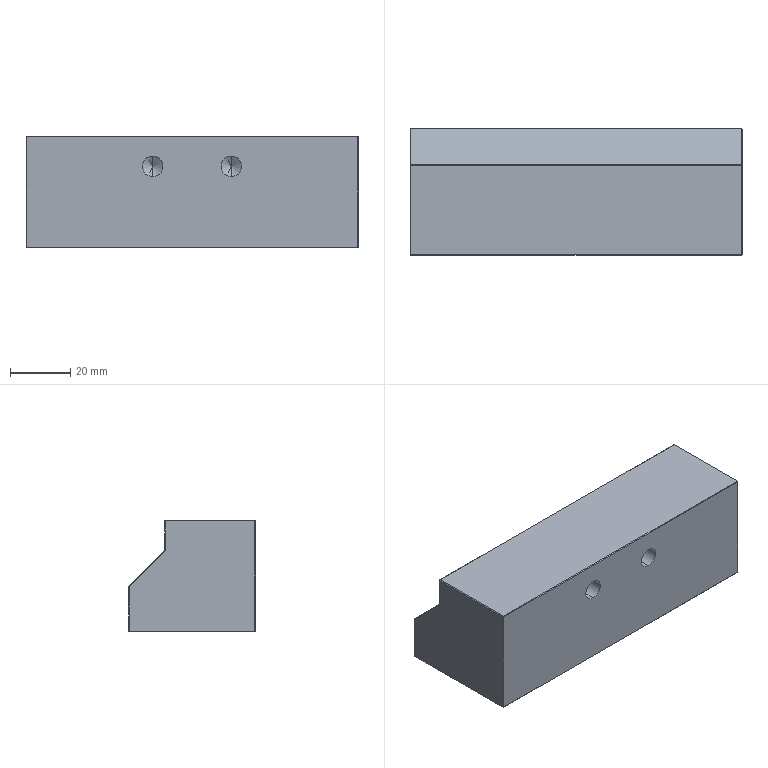Part | 1 solid | 40 faces | box 110 x 42 x 37 mm | volume 148303 mm3 | plane 32 | cylinder 4 | cone 4 | commonest cylinder face diameters 6.8 x4
STEP:
#1=CARTESIAN_POINT('',(-13.,20.,9.4));
#2=VERTEX_POINT('',#1);
#3=CARTESIAN_POINT('',(-13.,20.,2.6));
#4=VERTEX_POINT('',#3);
#5=CARTESIAN_POINT('',(-13.,20.,6.));
#6=DIRECTION('',(0.,-1.,0.));
#7=DIRECTION('',(0.,0.,-1.));
#8=AXIS2_PLACEMENT_3D('',#5,#6,#7);
#9=CIRCLE('',#8,3.4);
#10=EDGE_CURVE('',#2,#4,#9,.T.);
#11=ORIENTED_EDGE('',*,*,#10,.F.);
#12=CARTESIAN_POINT('',(-13.,0.,9.4));
#13=VERTEX_POINT('',#12);
#14=CARTESIAN_POINT('',(-13.,0.,9.4));
#15=DIRECTION('',(0.,-1.,0.));
#16=VECTOR('',#15,1000.);
#17=LINE('',#14,#16);
#18=EDGE_CURVE('',#2,#13,#17,.T.);
#19=ORIENTED_EDGE('',*,*,#18,.T.);
#20=CARTESIAN_POINT('',(-13.,0.,2.6));
#21=VERTEX_POINT('',#20);
#22=CARTESIAN_POINT('',(-13.,0.,6.));
#23=DIRECTION('',(0.,-1.,0.));
#24=DIRECTION('',(0.,0.,-1.));
#25=AXIS2_PLACEMENT_3D('',#22,#23,#24);
#26=CIRCLE('',#25,3.4);
#27=EDGE_CURVE('',#13,#21,#26,.T.);
#28=ORIENTED_EDGE('',*,*,#27,.T.);
#29=CARTESIAN_POINT('',(-13.,0.,2.6));
#30=DIRECTION('',(0.,-1.,0.));
#31=VECTOR('',#30,1000.);
#32=LINE('',#29,#31);
#33=EDGE_CURVE('',#4,#21,#32,.T.);
#34=ORIENTED_EDGE('',*,*,#33,.F.);
#35=EDGE_LOOP('',(#11,#19,#28,#34));
#36=FACE_OUTER_BOUND('',#35,.T.);
#37=CARTESIAN_POINT('',(-13.,0.,6.));
#38=DIRECTION('',(0.,-1.,0.));
#39=DIRECTION('',(0.,0.,-1.));
#40=AXIS2_PLACEMENT_3D('',#37,#38,#39);
#41=CYLINDRICAL_SURFACE('',#40,3.4);
#42=ADVANCED_FACE('',(#36),#41,.F.);
#43=CARTESIAN_POINT('',(-13.,22.043,6.));
#44=VERTEX_POINT('',#43);
#45=CARTESIAN_POINT('',(-13.,20.,2.6));
#46=DIRECTION('',(0.,-0.515,-0.8572));
#47=VECTOR('',#46,1000.);
#48=LINE('',#45,#47);
#49=EDGE_CURVE('',#44,#4,#48,.T.);
#50=ORIENTED_EDGE('',*,*,#49,.F.);
#51=CARTESIAN_POINT('',(-13.,20.,9.4));
#52=DIRECTION('',(0.,-0.515,0.8572));
#53=VECTOR('',#52,1000.);
#54=LINE('',#51,#53);
#55=EDGE_CURVE('',#44,#2,#54,.T.);
#56=ORIENTED_EDGE('',*,*,#55,.T.);
#57=ORIENTED_EDGE('',*,*,#10,.T.);
#58=EDGE_LOOP('',(#50,#56,#57));
#59=FACE_OUTER_BOUND('',#58,.T.);
#60=CARTESIAN_POINT('',(-13.,20.,6.));
#61=DIRECTION('',(0.,-1.,0.));
#62=DIRECTION('',(0.,0.,-1.));
#63=AXIS2_PLACEMENT_3D('',#60,#61,#62);
#64=CONICAL_SURFACE('',#63,3.4,1.03);
#65=ADVANCED_FACE('',(#59),#64,.F.);
#66=CARTESIAN_POINT('',(13.,20.,9.4));
#67=VERTEX_POINT('',#66);
#68=CARTESIAN_POINT('',(13.,20.,2.6));
#69=VERTEX_POINT('',#68);
#70=CARTESIAN_POINT('',(13.,20.,6.));
#71=DIRECTION('',(0.,-1.,0.));
#72=DIRECTION('',(0.,0.,-1.));
#73=AXIS2_PLACEMENT_3D('',#70,#71,#72);
#74=CIRCLE('',#73,3.4);
#75=EDGE_CURVE('',#67,#69,#74,.T.);
#76=ORIENTED_EDGE('',*,*,#75,.F.);
#77=CARTESIAN_POINT('',(13.,0.,9.4));
#78=VERTEX_POINT('',#77);
#79=CARTESIAN_POINT('',(13.,0.,9.4));
#80=DIRECTION('',(0.,-1.,0.));
#81=VECTOR('',#80,1000.);
#82=LINE('',#79,#81);
#83=EDGE_CURVE('',#67,#78,#82,.T.);
#84=ORIENTED_EDGE('',*,*,#83,.T.);
#85=CARTESIAN_POINT('',(13.,0.,2.6));
#86=VERTEX_POINT('',#85);
#87=CARTESIAN_POINT('',(13.,0.,6.));
#88=DIRECTION('',(0.,-1.,0.));
#89=DIRECTION('',(0.,0.,-1.));
#90=AXIS2_PLACEMENT_3D('',#87,#88,#89);
#91=CIRCLE('',#90,3.4);
#92=EDGE_CURVE('',#78,#86,#91,.T.);
#93=ORIENTED_EDGE('',*,*,#92,.T.);
#94=CARTESIAN_POINT('',(13.,0.,2.6));
#95=DIRECTION('',(0.,-1.,0.));
#96=VECTOR('',#95,1000.);
#97=LINE('',#94,#96);
#98=EDGE_CURVE('',#69,#86,#97,.T.);
#99=ORIENTED_EDGE('',*,*,#98,.F.);
#100=EDGE_LOOP('',(#76,#84,#93,#99));
#101=FACE_OUTER_BOUND('',#100,.T.);
#102=CARTESIAN_POINT('',(13.,0.,6.));
#103=DIRECTION('',(0.,-1.,0.));
#104=DIRECTION('',(0.,0.,-1.));
#105=AXIS2_PLACEMENT_3D('',#102,#103,#104);
#106=CYLINDRICAL_SURFACE('',#105,3.4);
#107=ADVANCED_FACE('',(#101),#106,.F.);
#108=CARTESIAN_POINT('',(13.,22.043,6.));
#109=VERTEX_POINT('',#108);
#110=CARTESIAN_POINT('',(13.,20.,2.6));
#111=DIRECTION('',(0.,-0.515,-0.8572));
#112=VECTOR('',#111,1000.);
#113=LINE('',#110,#112);
#114=EDGE_CURVE('',#109,#69,#113,.T.);
#115=ORIENTED_EDGE('',*,*,#114,.F.);
#116=CARTESIAN_POINT('',(13.,20.,9.4));
#117=DIRECTION('',(0.,-0.515,0.8572));
#118=VECTOR('',#117,1000.);
#119=LINE('',#116,#118);
#120=EDGE_CURVE('',#109,#67,#119,.T.);
#121=ORIENTED_EDGE('',*,*,#120,.T.);
#122=ORIENTED_EDGE('',*,*,#75,.T.);
#123=EDGE_LOOP('',(#115,#121,#122));
#124=FACE_OUTER_BOUND('',#123,.T.);
#125=CARTESIAN_POINT('',(13.,20.,6.));
#126=DIRECTION('',(0.,-1.,0.));
#127=DIRECTION('',(0.,0.,-1.));
#128=AXIS2_PLACEMENT_3D('',#125,#126,#127);
#129=CONICAL_SURFACE('',#128,3.4,1.03);
#130=ADVANCED_FACE('',(#124),#129,.F.);
#131=CARTESIAN_POINT('',(-54.8,0.,15.8));
#132=VERTEX_POINT('',#131);
#133=CARTESIAN_POINT('',(-54.8,0.,-20.8));
#134=VERTEX_POINT('',#133);
#135=CARTESIAN_POINT('',(-54.8,0.,10.));
#136=DIRECTION('',(0.,0.,-1.));
#137=VECTOR('',#136,1000.);
#138=LINE('',#135,#137);
#139=EDGE_CURVE('',#132,#134,#138,.T.);
#140=ORIENTED_EDGE('',*,*,#139,.T.);
#141=CARTESIAN_POINT('',(54.8,0.,-20.8));
#142=VERTEX_POINT('',#141);
#143=CARTESIAN_POINT('',(55.,0.,-20.8));
#144=DIRECTION('',(1.,0.,0.));
#145=VECTOR('',#144,1000.);
#146=LINE('',#143,#145);
#147=EDGE_CURVE('',#134,#142,#146,.T.);
#148=ORIENTED_EDGE('',*,*,#147,.T.);
#149=CARTESIAN_POINT('',(54.8,0.,15.8));
#150=VERTEX_POINT('',#149);
#151=CARTESIAN_POINT('',(54.8,0.,16.));
#152=DIRECTION('',(0.,0.,1.));
#153=VECTOR('',#152,1000.);
#154=LINE('',#151,#153);
#155=EDGE_CURVE('',#142,#150,#154,.T.);
#156=ORIENTED_EDGE('',*,*,#155,.T.);
#157=CARTESIAN_POINT('',(55.,0.,15.8));
#158=DIRECTION('',(-1.,0.,0.));
#159=VECTOR('',#158,1000.);
#160=LINE('',#157,#159);
#161=EDGE_CURVE('',#150,#132,#160,.T.);
#162=ORIENTED_EDGE('',*,*,#161,.T.);
#163=EDGE_LOOP('',(#140,#148,#156,#162));
#164=FACE_OUTER_BOUND('',#163,.T.);
#165=CARTESIAN_POINT('',(-13.,0.,6.));
#166=DIRECTION('',(0.,-1.,0.));
#167=DIRECTION('',(0.,0.,-1.));
#168=AXIS2_PLACEMENT_3D('',#165,#166,#167);
#169=CIRCLE('',#168,3.4);
#170=EDGE_CURVE('',#21,#13,#169,.T.);
#171=ORIENTED_EDGE('',*,*,#170,.F.);
#172=ORIENTED_EDGE('',*,*,#27,.F.);
#173=EDGE_LOOP('',(#171,#172));
#174=FACE_BOUND('',#173,.T.);
#175=CARTESIAN_POINT('',(13.,0.,6.));
#176=DIRECTION('',(0.,-1.,0.));
#177=DIRECTION('',(0.,0.,-1.));
#178=AXIS2_PLACEMENT_3D('',#175,#176,#177);
#179=CIRCLE('',#178,3.4);
#180=EDGE_CURVE('',#86,#78,#179,.T.);
#181=ORIENTED_EDGE('',*,*,#180,.F.);
#182=ORIENTED_EDGE('',*,*,#92,.F.);
#183=EDGE_LOOP('',(#181,#182));
#184=FACE_BOUND('',#183,.T.);
#185=CARTESIAN_POINT('',(55.,0.,10.));
#186=DIRECTION('',(0.,1.,0.));
#187=DIRECTION('',(0.,0.,1.));
#188=AXIS2_PLACEMENT_3D('',#185,#186,#187);
#189=PLANE('',#188);
#190=ADVANCED_FACE('',(#164,#174,#184),#189,.F.);
#191=CARTESIAN_POINT('',(-54.8,41.8,-21.));
#192=VERTEX_POINT('',#191);
#193=CARTESIAN_POINT('',(54.8,41.8,-21.));
#194=VERTEX_POINT('',#193);
#195=CARTESIAN_POINT('',(55.,41.8,-21.));
#196=DIRECTION('',(1.,0.,0.));
#197=VECTOR('',#196,1000.);
#198=LINE('',#195,#197);
#199=EDGE_CURVE('',#192,#194,#198,.T.);
#200=ORIENTED_EDGE('',*,*,#199,.T.);
#201=CARTESIAN_POINT('',(54.8,0.2,-21.));
#202=VERTEX_POINT('',#201);
#203=CARTESIAN_POINT('',(54.8,0.,-21.));
#204=DIRECTION('',(0.,-1.,0.));
#205=VECTOR('',#204,1000.);
#206=LINE('',#203,#205);
#207=EDGE_CURVE('',#194,#202,#206,.T.);
#208=ORIENTED_EDGE('',*,*,#207,.T.);
#209=CARTESIAN_POINT('',(-54.8,0.2,-21.));
#210=VERTEX_POINT('',#209);
#211=CARTESIAN_POINT('',(55.,0.2,-21.));
#212=DIRECTION('',(-1.,0.,0.));
#213=VECTOR('',#212,1000.);
#214=LINE('',#211,#213);
#215=EDGE_CURVE('',#202,#210,#214,.T.);
#216=ORIENTED_EDGE('',*,*,#215,.T.);
#217=CARTESIAN_POINT('',(-54.8,0.,-21.));
#218=DIRECTION('',(0.,1.,0.));
#219=VECTOR('',#218,1000.);
#220=LINE('',#217,#219);
#221=EDGE_CURVE('',#210,#192,#220,.T.);
#222=ORIENTED_EDGE('',*,*,#221,.T.);
#223=EDGE_LOOP('',(#200,#208,#216,#222));
#224=FACE_OUTER_BOUND('',#223,.T.);
#225=CARTESIAN_POINT('',(55.,0.,-21.));
#226=DIRECTION('',(0.,0.,1.));
#227=DIRECTION('',(1.,0.,0.));
#228=AXIS2_PLACEMENT_3D('',#225,#226,#227);
#229=PLANE('',#228);
#230=ADVANCED_FACE('',(#224),#229,.F.);
#231=CARTESIAN_POINT('',(54.8,42.,-6.));
#232=VERTEX_POINT('',#231);
#233=CARTESIAN_POINT('',(-54.8,42.,-6.));
#234=VERTEX_POINT('',#233);
#235=CARTESIAN_POINT('',(55.,42.,-6.));
#236=DIRECTION('',(-1.,0.,0.));
#237=VECTOR('',#236,1000.);
#238=LINE('',#235,#237);
#239=EDGE_CURVE('',#232,#234,#238,.T.);
#240=ORIENTED_EDGE('',*,*,#239,.F.);
#241=CARTESIAN_POINT('',(54.8,42.,-20.8));
#242=VERTEX_POINT('',#241);
#243=CARTESIAN_POINT('',(54.8,42.,-21.));
#244=DIRECTION('',(0.,0.,-1.));
#245=VECTOR('',#244,1000.);
#246=LINE('',#243,#245);
#247=EDGE_CURVE('',#232,#242,#246,.T.);
#248=ORIENTED_EDGE('',*,*,#247,.T.);
#249=CARTESIAN_POINT('',(-54.8,42.,-20.8));
#250=VERTEX_POINT('',#249);
#251=CARTESIAN_POINT('',(55.,42.,-20.8));
#252=DIRECTION('',(-1.,0.,0.));
#253=VECTOR('',#252,1000.);
#254=LINE('',#251,#253);
#255=EDGE_CURVE('',#242,#250,#254,.T.);
#256=ORIENTED_EDGE('',*,*,#255,.T.);
#257=CARTESIAN_POINT('',(-54.8,42.,-21.));
#258=DIRECTION('',(0.,0.,1.));
#259=VECTOR('',#258,1000.);
#260=LINE('',#257,#259);
#261=EDGE_CURVE('',#250,#234,#260,.T.);
#262=ORIENTED_EDGE('',*,*,#261,.T.);
#263=EDGE_LOOP('',(#240,#248,#256,#262));
#264=FACE_OUTER_BOUND('',#263,.T.);
#265=CARTESIAN_POINT('',(55.,42.,-21.));
#266=DIRECTION('',(0.,-1.,0.));
#267=DIRECTION('',(0.,0.,-1.));
#268=AXIS2_PLACEMENT_3D('',#265,#266,#267);
#269=PLANE('',#268);
#270=ADVANCED_FACE('',(#264),#269,.F.);
#271=CARTESIAN_POINT('',(54.8,30.,6.));
#272=VERTEX_POINT('',#271);
#273=CARTESIAN_POINT('',(-54.8,30.,6.));
#274=VERTEX_POINT('',#273);
#275=CARTESIAN_POINT('',(55.,30.,6.));
#276=DIRECTION('',(-1.,0.,0.));
#277=VECTOR('',#276,1000.);
#278=LINE('',#275,#277);
#279=EDGE_CURVE('',#272,#274,#278,.T.);
#280=ORIENTED_EDGE('',*,*,#279,.F.);
#281=CARTESIAN_POINT('',(54.8,42.,-6.));
#282=DIRECTION('',(0.,0.7071,-0.7071));
#283=VECTOR('',#282,1000.);
#284=LINE('',#281,#283);
#285=EDGE_CURVE('',#272,#232,#284,.T.);
#286=ORIENTED_EDGE('',*,*,#285,.T.);
#287=ORIENTED_EDGE('',*,*,#239,.T.);
#288=CARTESIAN_POINT('',(-54.8,42.,-6.));
#289=DIRECTION('',(0.,-0.7071,0.7071));
#290=VECTOR('',#289,1000.);
#291=LINE('',#288,#290);
#292=EDGE_CURVE('',#234,#274,#291,.T.);
#293=ORIENTED_EDGE('',*,*,#292,.T.);
#294=EDGE_LOOP('',(#280,#286,#287,#293));
#295=FACE_OUTER_BOUND('',#294,.T.);
#296=CARTESIAN_POINT('',(55.,42.,-6.));
#297=DIRECTION('',(0.,-0.7071,-0.7071));
#298=DIRECTION('',(0.,0.7071,-0.7071));
#299=AXIS2_PLACEMENT_3D('',#296,#297,#298);
#300=PLANE('',#299);
#301=ADVANCED_FACE('',(#295),#300,.F.);
#302=CARTESIAN_POINT('',(-54.8,30.,15.8));
#303=VERTEX_POINT('',#302);
#304=CARTESIAN_POINT('',(54.8,30.,15.8));
#305=VERTEX_POINT('',#304);
#306=CARTESIAN_POINT('',(55.,30.,15.8));
#307=DIRECTION('',(1.,0.,0.));
#308=VECTOR('',#307,1000.);
#309=LINE('',#306,#308);
#310=EDGE_CURVE('',#303,#305,#309,.T.);
#311=ORIENTED_EDGE('',*,*,#310,.T.);
#312=CARTESIAN_POINT('',(54.8,30.,6.));
#313=DIRECTION('',(0.,0.,-1.));
#314=VECTOR('',#313,1000.);
#315=LINE('',#312,#314);
#316=EDGE_CURVE('',#305,#272,#315,.T.);
#317=ORIENTED_EDGE('',*,*,#316,.T.);
#318=ORIENTED_EDGE('',*,*,#279,.T.);
#319=CARTESIAN_POINT('',(-54.8,30.,6.));
#320=DIRECTION('',(0.,0.,1.));
#321=VECTOR('',#320,1000.);
#322=LINE('',#319,#321);
#323=EDGE_CURVE('',#274,#303,#322,.T.);
#324=ORIENTED_EDGE('',*,*,#323,.T.);
#325=EDGE_LOOP('',(#311,#317,#318,#324));
#326=FACE_OUTER_BOUND('',#325,.T.);
#327=CARTESIAN_POINT('',(55.,30.,6.));
#328=DIRECTION('',(0.,-1.,0.));
#329=DIRECTION('',(0.,0.,-1.));
#330=AXIS2_PLACEMENT_3D('',#327,#328,#329);
#331=PLANE('',#330);
#332=ADVANCED_FACE('',(#326),#331,.F.);
#333=CARTESIAN_POINT('',(54.8,0.2,16.));
#334=VERTEX_POINT('',#333);
#335=CARTESIAN_POINT('',(54.8,29.8,16.));
#336=VERTEX_POINT('',#335);
#337=CARTESIAN_POINT('',(54.8,30.,16.));
#338=DIRECTION('',(0.,1.,0.));
#339=VECTOR('',#338,1000.);
#340=LINE('',#337,#339);
#341=EDGE_CURVE('',#334,#336,#340,.T.);
#342=ORIENTED_EDGE('',*,*,#341,.T.);
#343=CARTESIAN_POINT('',(-54.8,29.8,16.));
#344=VERTEX_POINT('',#343);
#345=CARTESIAN_POINT('',(55.,29.8,16.));
#346=DIRECTION('',(-1.,0.,0.));
#347=VECTOR('',#346,1000.);
#348=LINE('',#345,#347);
#349=EDGE_CURVE('',#336,#344,#348,.T.);
#350=ORIENTED_EDGE('',*,*,#349,.T.);
#351=CARTESIAN_POINT('',(-54.8,0.2,16.));
#352=VERTEX_POINT('',#351);
#353=CARTESIAN_POINT('',(-54.8,30.,16.));
#354=DIRECTION('',(0.,-1.,0.));
#355=VECTOR('',#354,1000.);
#356=LINE('',#353,#355);
#357=EDGE_CURVE('',#344,#352,#356,.T.);
#358=ORIENTED_EDGE('',*,*,#357,.T.);
#359=CARTESIAN_POINT('',(55.,0.2,16.));
#360=DIRECTION('',(1.,0.,0.));
#361=VECTOR('',#360,1000.);
#362=LINE('',#359,#361);
#363=EDGE_CURVE('',#352,#334,#362,.T.);
#364=ORIENTED_EDGE('',*,*,#363,.T.);
#365=EDGE_LOOP('',(#342,#350,#358,#364));
#366=FACE_OUTER_BOUND('',#365,.T.);
#367=CARTESIAN_POINT('',(55.,30.,16.));
#368=DIRECTION('',(0.,0.,-1.));
#369=DIRECTION('',(0.,1.,0.));
#370=AXIS2_PLACEMENT_3D('',#367,#368,#369);
#371=PLANE('',#370);
#372=ADVANCED_FACE('',(#366),#371,.F.);
#373=CARTESIAN_POINT('',(55.,29.8,5.917));
#374=VERTEX_POINT('',#373);
#375=CARTESIAN_POINT('',(55.,29.8,15.8));
#376=VERTEX_POINT('',#375);
#377=CARTESIAN_POINT('',(55.,29.8,16.));
#378=DIRECTION('',(0.,0.,1.));
#379=VECTOR('',#378,1000.);
#380=LINE('',#377,#379);
#381=EDGE_CURVE('',#374,#376,#380,.T.);
#382=ORIENTED_EDGE('',*,*,#381,.T.);
#383=CARTESIAN_POINT('',(55.,0.2,15.8));
#384=VERTEX_POINT('',#383);
#385=CARTESIAN_POINT('',(55.,0.,15.8));
#386=DIRECTION('',(0.,-1.,0.));
#387=VECTOR('',#386,1000.);
#388=LINE('',#385,#387);
#389=EDGE_CURVE('',#376,#384,#388,.T.);
#390=ORIENTED_EDGE('',*,*,#389,.T.);
#391=CARTESIAN_POINT('',(55.,0.2,-20.8));
#392=VERTEX_POINT('',#391);
#393=CARTESIAN_POINT('',(55.,0.2,-21.));
#394=DIRECTION('',(0.,0.,-1.));
#395=VECTOR('',#394,1000.);
#396=LINE('',#393,#395);
#397=EDGE_CURVE('',#384,#392,#396,.T.);
#398=ORIENTED_EDGE('',*,*,#397,.T.);
#399=CARTESIAN_POINT('',(55.,41.8,-20.8));
#400=VERTEX_POINT('',#399);
#401=CARTESIAN_POINT('',(55.,42.,-20.8));
#402=DIRECTION('',(0.,1.,0.));
#403=VECTOR('',#402,1000.);
#404=LINE('',#401,#403);
#405=EDGE_CURVE('',#392,#400,#404,.T.);
#406=ORIENTED_EDGE('',*,*,#405,.T.);
#407=CARTESIAN_POINT('',(55.,41.8,-6.083));
#408=VERTEX_POINT('',#407);
#409=CARTESIAN_POINT('',(55.,41.8,-6.));
#410=DIRECTION('',(0.,0.,1.));
#411=VECTOR('',#410,1000.);
#412=LINE('',#409,#411);
#413=EDGE_CURVE('',#400,#408,#412,.T.);
#414=ORIENTED_EDGE('',*,*,#413,.T.);
#415=CARTESIAN_POINT('',(55.,29.859,5.859));
#416=DIRECTION('',(0.,-0.7071,0.7071));
#417=VECTOR('',#416,1000.);
#418=LINE('',#415,#417);
#419=EDGE_CURVE('',#408,#374,#418,.T.);
#420=ORIENTED_EDGE('',*,*,#419,.T.);
#421=EDGE_LOOP('',(#382,#390,#398,#406,#414,#420));
#422=FACE_OUTER_BOUND('',#421,.T.);
#423=CARTESIAN_POINT('',(55.,0.,0.));
#424=DIRECTION('',(1.,0.,0.));
#425=DIRECTION('',(0.,0.,-1.));
#426=AXIS2_PLACEMENT_3D('',#423,#424,#425);
#427=PLANE('',#426);
#428=ADVANCED_FACE('',(#422),#427,.T.);
#429=CARTESIAN_POINT('',(-55.,0.2,-20.8));
#430=VERTEX_POINT('',#429);
#431=CARTESIAN_POINT('',(-55.,0.2,15.8));
#432=VERTEX_POINT('',#431);
#433=CARTESIAN_POINT('',(-55.,0.2,0.));
#434=DIRECTION('',(0.,0.,1.));
#435=VECTOR('',#434,1000.);
#436=LINE('',#433,#435);
#437=EDGE_CURVE('',#430,#432,#436,.T.);
#438=ORIENTED_EDGE('',*,*,#437,.T.);
#439=CARTESIAN_POINT('',(-55.,29.8,15.8));
#440=VERTEX_POINT('',#439);
#441=CARTESIAN_POINT('',(-55.,0.,15.8));
#442=DIRECTION('',(0.,1.,0.));
#443=VECTOR('',#442,1000.);
#444=LINE('',#441,#443);
#445=EDGE_CURVE('',#432,#440,#444,.T.);
#446=ORIENTED_EDGE('',*,*,#445,.T.);
#447=CARTESIAN_POINT('',(-55.,29.8,5.917));
#448=VERTEX_POINT('',#447);
#449=CARTESIAN_POINT('',(-55.,29.8,0.));
#450=DIRECTION('',(0.,0.,-1.));
#451=VECTOR('',#450,1000.);
#452=LINE('',#449,#451);
#453=EDGE_CURVE('',#440,#448,#452,.T.);
#454=ORIENTED_EDGE('',*,*,#453,.T.);
#455=CARTESIAN_POINT('',(-55.,41.8,-6.083));
#456=VERTEX_POINT('',#455);
#457=CARTESIAN_POINT('',(-55.,17.859,17.859));
#458=DIRECTION('',(0.,0.7071,-0.7071));
#459=VECTOR('',#458,1000.);
#460=LINE('',#457,#459);
#461=EDGE_CURVE('',#448,#456,#460,.T.);
#462=ORIENTED_EDGE('',*,*,#461,.T.);
#463=CARTESIAN_POINT('',(-55.,41.8,-20.8));
#464=VERTEX_POINT('',#463);
#465=CARTESIAN_POINT('',(-55.,41.8,0.));
#466=DIRECTION('',(0.,0.,-1.));
#467=VECTOR('',#466,1000.);
#468=LINE('',#465,#467);
#469=EDGE_CURVE('',#456,#464,#468,.T.);
#470=ORIENTED_EDGE('',*,*,#469,.T.);
#471=CARTESIAN_POINT('',(-55.,0.,-20.8));
#472=DIRECTION('',(0.,-1.,0.));
#473=VECTOR('',#472,1000.);
#474=LINE('',#471,#473);
#475=EDGE_CURVE('',#464,#430,#474,.T.);
#476=ORIENTED_EDGE('',*,*,#475,.T.);
#477=EDGE_LOOP('',(#438,#446,#454,#462,#470,#476));
#478=FACE_OUTER_BOUND('',#477,.T.);
#479=CARTESIAN_POINT('',(-55.,0.,0.));
#480=DIRECTION('',(1.,0.,0.));
#481=DIRECTION('',(0.,0.,-1.));
#482=AXIS2_PLACEMENT_3D('',#479,#480,#481);
#483=PLANE('',#482);
#484=ADVANCED_FACE('',(#478),#483,.F.);
#485=ORIENTED_EDGE('',*,*,#120,.F.);
#486=ORIENTED_EDGE('',*,*,#114,.T.);
#487=CARTESIAN_POINT('',(13.,20.,6.));
#488=DIRECTION('',(0.,-1.,0.));
#489=DIRECTION('',(0.,0.,-1.));
#490=AXIS2_PLACEMENT_3D('',#487,#488,#489);
#491=CIRCLE('',#490,3.4);
#492=EDGE_CURVE('',#69,#67,#491,.T.);
#493=ORIENTED_EDGE('',*,*,#492,.T.);
#494=EDGE_LOOP('',(#485,#486,#493));
#495=FACE_OUTER_BOUND('',#494,.T.);
#496=CARTESIAN_POINT('',(13.,20.,6.));
#497=DIRECTION('',(0.,-1.,0.));
#498=DIRECTION('',(0.,0.,-1.));
#499=AXIS2_PLACEMENT_3D('',#496,#497,#498);
#500=CONICAL_SURFACE('',#499,3.4,1.03);
#501=ADVANCED_FACE('',(#495),#500,.F.);
#502=ORIENTED_EDGE('',*,*,#83,.F.);
#503=ORIENTED_EDGE('',*,*,#492,.F.);
#504=ORIENTED_EDGE('',*,*,#98,.T.);
#505=ORIENTED_EDGE('',*,*,#180,.T.);
#506=EDGE_LOOP('',(#502,#503,#504,#505));
#507=FACE_OUTER_BOUND('',#506,.T.);
#508=CARTESIAN_POINT('',(13.,0.,6.));
#509=DIRECTION('',(0.,-1.,0.));
#510=DIRECTION('',(0.,0.,-1.));
#511=AXIS2_PLACEMENT_3D('',#508,#509,#510);
#512=CYLINDRICAL_SURFACE('',#511,3.4);
#513=ADVANCED_FACE('',(#507),#512,.F.);
#514=ORIENTED_EDGE('',*,*,#55,.F.);
#515=ORIENTED_EDGE('',*,*,#49,.T.);
#516=CARTESIAN_POINT('',(-13.,20.,6.));
#517=DIRECTION('',(0.,-1.,0.));
#518=DIRECTION('',(0.,0.,-1.));
#519=AXIS2_PLACEMENT_3D('',#516,#517,#518);
#520=CIRCLE('',#519,3.4);
#521=EDGE_CURVE('',#4,#2,#520,.T.);
#522=ORIENTED_EDGE('',*,*,#521,.T.);
#523=EDGE_LOOP('',(#514,#515,#522));
#524=FACE_OUTER_BOUND('',#523,.T.);
#525=CARTESIAN_POINT('',(-13.,20.,6.));
#526=DIRECTION('',(0.,-1.,0.));
#527=DIRECTION('',(0.,0.,-1.));
#528=AXIS2_PLACEMENT_3D('',#525,#526,#527);
#529=CONICAL_SURFACE('',#528,3.4,1.03);
#530=ADVANCED_FACE('',(#524),#529,.F.);
#531=ORIENTED_EDGE('',*,*,#18,.F.);
#532=ORIENTED_EDGE('',*,*,#521,.F.);
#533=ORIENTED_EDGE('',*,*,#33,.T.);
#534=ORIENTED_EDGE('',*,*,#170,.T.);
#535=EDGE_LOOP('',(#531,#532,#533,#534));
#536=FACE_OUTER_BOUND('',#535,.T.);
#537=CARTESIAN_POINT('',(-13.,0.,6.));
#538=DIRECTION('',(0.,-1.,0.));
#539=DIRECTION('',(0.,0.,-1.));
#540=AXIS2_PLACEMENT_3D('',#537,#538,#539);
#541=CYLINDRICAL_SURFACE('',#540,3.4);
#542=ADVANCED_FACE('',(#536),#541,.F.);
#543=CARTESIAN_POINT('',(56.129,28.671,5.45));
#544=DIRECTION('',(0.6786,-0.6786,-0.2811));
#545=VECTOR('',#544,1000.);
#546=LINE('',#543,#545);
#547=EDGE_CURVE('',#272,#374,#546,.T.);
#548=ORIENTED_EDGE('',*,*,#547,.F.);
#549=ORIENTED_EDGE('',*,*,#316,.F.);
#550=CARTESIAN_POINT('',(54.8,30.,15.8));
#551=DIRECTION('',(-0.7071,0.7071,0.));
#552=VECTOR('',#551,1000.);
#553=LINE('',#550,#552);
#554=EDGE_CURVE('',#376,#305,#553,.T.);
#555=ORIENTED_EDGE('',*,*,#554,.F.);
#556=ORIENTED_EDGE('',*,*,#381,.F.);
#557=EDGE_LOOP('',(#548,#549,#555,#556));
#558=FACE_OUTER_BOUND('',#557,.T.);
#559=CARTESIAN_POINT('',(55.,29.8,0.));
#560=DIRECTION('',(0.7071,0.7071,0.));
#561=DIRECTION('',(0.,0.,-1.));
#562=AXIS2_PLACEMENT_3D('',#559,#560,#561);
#563=PLANE('',#562);
#564=ADVANCED_FACE('',(#558),#563,.T.);
#565=CARTESIAN_POINT('',(-54.9,29.9,15.8));
#566=DIRECTION('',(-0.7071,-0.7071,0.));
#567=VECTOR('',#566,1000.);
#568=LINE('',#565,#567);
#569=EDGE_CURVE('',#303,#440,#568,.T.);
#570=ORIENTED_EDGE('',*,*,#569,.F.);
#571=ORIENTED_EDGE('',*,*,#323,.F.);
#572=CARTESIAN_POINT('',(-54.8,30.,6.));
#573=DIRECTION('',(0.6786,0.6786,0.2811));
#574=VECTOR('',#573,1000.);
#575=LINE('',#572,#574);
#576=EDGE_CURVE('',#448,#274,#575,.T.);
#577=ORIENTED_EDGE('',*,*,#576,.F.);
#578=ORIENTED_EDGE('',*,*,#453,.F.);
#579=EDGE_LOOP('',(#570,#571,#577,#578));
#580=FACE_OUTER_BOUND('',#579,.T.);
#581=CARTESIAN_POINT('',(-54.8,30.,6.));
#582=DIRECTION('',(0.7071,-0.7071,0.));
#583=DIRECTION('',(0.,0.,1.));
#584=AXIS2_PLACEMENT_3D('',#581,#582,#583);
#585=PLANE('',#584);
#586=ADVANCED_FACE('',(#580),#585,.F.);
#587=CARTESIAN_POINT('',(54.8,30.,15.8));
#588=DIRECTION('',(0.,-0.7071,0.7071));
#589=VECTOR('',#588,1000.);
#590=LINE('',#587,#589);
#591=EDGE_CURVE('',#305,#336,#590,.T.);
#592=ORIENTED_EDGE('',*,*,#591,.F.);
#593=ORIENTED_EDGE('',*,*,#310,.F.);
#594=CARTESIAN_POINT('',(-54.8,29.8,16.));
#595=DIRECTION('',(0.,0.7071,-0.7071));
#596=VECTOR('',#595,1000.);
#597=LINE('',#594,#596);
#598=EDGE_CURVE('',#344,#303,#597,.T.);
#599=ORIENTED_EDGE('',*,*,#598,.F.);
#600=ORIENTED_EDGE('',*,*,#349,.F.);
#601=EDGE_LOOP('',(#592,#593,#599,#600));
#602=FACE_OUTER_BOUND('',#601,.T.);
#603=CARTESIAN_POINT('',(55.,29.8,16.));
#604=DIRECTION('',(0.,-0.7071,-0.7071));
#605=DIRECTION('',(-1.,0.,0.));
#606=AXIS2_PLACEMENT_3D('',#603,#604,#605);
#607=PLANE('',#606);
#608=ADVANCED_FACE('',(#602),#607,.F.);
#609=ORIENTED_EDGE('',*,*,#554,.T.);
#610=ORIENTED_EDGE('',*,*,#591,.T.);
#611=CARTESIAN_POINT('',(54.9,29.8,15.9));
#612=DIRECTION('',(-0.7071,0.,0.7071));
#613=VECTOR('',#612,1000.);
#614=LINE('',#611,#613);
#615=EDGE_CURVE('',#376,#336,#614,.T.);
#616=ORIENTED_EDGE('',*,*,#615,.F.);
#617=EDGE_LOOP('',(#609,#610,#616));
#618=FACE_OUTER_BOUND('',#617,.T.);
#619=CARTESIAN_POINT('',(54.8,30.,15.8));
#620=DIRECTION('',(0.5774,0.5774,0.5774));
#621=DIRECTION('',(0.,-0.7071,0.7071));
#622=AXIS2_PLACEMENT_3D('',#619,#620,#621);
#623=PLANE('',#622);
#624=ADVANCED_FACE('',(#618),#623,.T.);
#625=ORIENTED_EDGE('',*,*,#547,.T.);
#626=ORIENTED_EDGE('',*,*,#419,.F.);
#627=CARTESIAN_POINT('',(53.84,42.96,-5.602));
#628=DIRECTION('',(0.6786,-0.6786,-0.2811));
#629=VECTOR('',#628,1000.);
#630=LINE('',#627,#629);
#631=EDGE_CURVE('',#232,#408,#630,.T.);
#632=ORIENTED_EDGE('',*,*,#631,.F.);
#633=ORIENTED_EDGE('',*,*,#285,.F.);
#634=EDGE_LOOP('',(#625,#626,#632,#633));
#635=FACE_OUTER_BOUND('',#634,.T.);
#636=CARTESIAN_POINT('',(55.,17.859,17.859));
#637=DIRECTION('',(0.7071,0.5,0.5));
#638=DIRECTION('',(0.,0.7071,-0.7071));
#639=AXIS2_PLACEMENT_3D('',#636,#637,#638);
#640=PLANE('',#639);
#641=ADVANCED_FACE('',(#635),#640,.T.);
#642=ORIENTED_EDGE('',*,*,#576,.T.);
#643=ORIENTED_EDGE('',*,*,#292,.F.);
#644=CARTESIAN_POINT('',(-57.661,39.139,-7.185));
#645=DIRECTION('',(0.6786,0.6786,0.2811));
#646=VECTOR('',#645,1000.);
#647=LINE('',#644,#646);
#648=EDGE_CURVE('',#456,#234,#647,.T.);
#649=ORIENTED_EDGE('',*,*,#648,.F.);
#650=ORIENTED_EDGE('',*,*,#461,.F.);
#651=EDGE_LOOP('',(#642,#643,#649,#650));
#652=FACE_OUTER_BOUND('',#651,.T.);
#653=CARTESIAN_POINT('',(-54.8,42.,-6.));
#654=DIRECTION('',(0.7071,-0.5,-0.5));
#655=DIRECTION('',(0.,-0.7071,0.7071));
#656=AXIS2_PLACEMENT_3D('',#653,#654,#655);
#657=PLANE('',#656);
#658=ADVANCED_FACE('',(#652),#657,.F.);
#659=ORIENTED_EDGE('',*,*,#598,.T.);
#660=ORIENTED_EDGE('',*,*,#569,.T.);
#661=CARTESIAN_POINT('',(-54.8,29.8,16.));
#662=DIRECTION('',(-0.7071,0.,-0.7071));
#663=VECTOR('',#662,1000.);
#664=LINE('',#661,#663);
#665=EDGE_CURVE('',#344,#440,#664,.T.);
#666=ORIENTED_EDGE('',*,*,#665,.F.);
#667=EDGE_LOOP('',(#659,#660,#666));
#668=FACE_OUTER_BOUND('',#667,.T.);
#669=CARTESIAN_POINT('',(-54.8,29.8,16.));
#670=DIRECTION('',(-0.5774,0.5774,0.5774));
#671=DIRECTION('',(-0.7071,-0.7071,0.));
#672=AXIS2_PLACEMENT_3D('',#669,#670,#671);
#673=PLANE('',#672);
#674=ADVANCED_FACE('',(#668),#673,.T.);
#675=ORIENTED_EDGE('',*,*,#615,.T.);
#676=ORIENTED_EDGE('',*,*,#341,.F.);
#677=CARTESIAN_POINT('',(55.,0.2,15.8));
#678=DIRECTION('',(-0.7071,0.,0.7071));
#679=VECTOR('',#678,1000.);
#680=LINE('',#677,#679);
#681=EDGE_CURVE('',#384,#334,#680,.T.);
#682=ORIENTED_EDGE('',*,*,#681,.F.);
#683=ORIENTED_EDGE('',*,*,#389,.F.);
#684=EDGE_LOOP('',(#675,#676,#682,#683));
#685=FACE_OUTER_BOUND('',#684,.T.);
#686=CARTESIAN_POINT('',(55.,0.,15.8));
#687=DIRECTION('',(0.7071,0.,0.7071));
#688=DIRECTION('',(0.,1.,0.));
#689=AXIS2_PLACEMENT_3D('',#686,#687,#688);
#690=PLANE('',#689);
#691=ADVANCED_FACE('',(#685),#690,.T.);
#692=ORIENTED_EDGE('',*,*,#631,.T.);
#693=ORIENTED_EDGE('',*,*,#413,.F.);
#694=CARTESIAN_POINT('',(54.9,41.9,-20.8));
#695=DIRECTION('',(0.7071,-0.7071,0.));
#696=VECTOR('',#695,1000.);
#697=LINE('',#694,#696);
#698=EDGE_CURVE('',#242,#400,#697,.T.);
#699=ORIENTED_EDGE('',*,*,#698,.F.);
#700=ORIENTED_EDGE('',*,*,#247,.F.);
#701=EDGE_LOOP('',(#692,#693,#699,#700));
#702=FACE_OUTER_BOUND('',#701,.T.);
#703=CARTESIAN_POINT('',(55.,41.8,0.));
#704=DIRECTION('',(0.7071,0.7071,0.));
#705=DIRECTION('',(0.,0.,-1.));
#706=AXIS2_PLACEMENT_3D('',#703,#704,#705);
#707=PLANE('',#706);
#708=ADVANCED_FACE('',(#702),#707,.T.);
#709=CARTESIAN_POINT('',(-54.8,42.,-20.8));
#710=DIRECTION('',(0.,-0.7071,-0.7071));
#711=VECTOR('',#710,1000.);
#712=LINE('',#709,#711);
#713=EDGE_CURVE('',#250,#192,#712,.T.);
#714=ORIENTED_EDGE('',*,*,#713,.F.);
#715=ORIENTED_EDGE('',*,*,#255,.F.);
#716=CARTESIAN_POINT('',(54.8,41.8,-21.));
#717=DIRECTION('',(0.,0.7071,0.7071));
#718=VECTOR('',#717,1000.);
#719=LINE('',#716,#718);
#720=EDGE_CURVE('',#194,#242,#719,.T.);
#721=ORIENTED_EDGE('',*,*,#720,.F.);
#722=ORIENTED_EDGE('',*,*,#199,.F.);
#723=EDGE_LOOP('',(#714,#715,#721,#722));
#724=FACE_OUTER_BOUND('',#723,.T.);
#725=CARTESIAN_POINT('',(55.,42.,-20.8));
#726=DIRECTION('',(0.,-0.7071,0.7071));
#727=DIRECTION('',(-1.,0.,0.));
#728=AXIS2_PLACEMENT_3D('',#725,#726,#727);
#729=PLANE('',#728);
#730=ADVANCED_FACE('',(#724),#729,.F.);
#731=ORIENTED_EDGE('',*,*,#648,.T.);
#732=ORIENTED_EDGE('',*,*,#261,.F.);
#733=CARTESIAN_POINT('',(-54.8,42.,-20.8));
#734=DIRECTION('',(0.7071,0.7071,0.));
#735=VECTOR('',#734,1000.);
#736=LINE('',#733,#735);
#737=EDGE_CURVE('',#464,#250,#736,.T.);
#738=ORIENTED_EDGE('',*,*,#737,.F.);
#739=ORIENTED_EDGE('',*,*,#469,.F.);
#740=EDGE_LOOP('',(#731,#732,#738,#739));
#741=FACE_OUTER_BOUND('',#740,.T.);
#742=CARTESIAN_POINT('',(-54.8,42.,-21.));
#743=DIRECTION('',(0.7071,-0.7071,0.));
#744=DIRECTION('',(0.,0.,1.));
#745=AXIS2_PLACEMENT_3D('',#742,#743,#744);
#746=PLANE('',#745);
#747=ADVANCED_FACE('',(#741),#746,.F.);
#748=ORIENTED_EDGE('',*,*,#665,.T.);
#749=ORIENTED_EDGE('',*,*,#445,.F.);
#750=CARTESIAN_POINT('',(-54.9,0.2,15.9));
#751=DIRECTION('',(-0.7071,0.,-0.7071));
#752=VECTOR('',#751,1000.);
#753=LINE('',#750,#752);
#754=EDGE_CURVE('',#352,#432,#753,.T.);
#755=ORIENTED_EDGE('',*,*,#754,.F.);
#756=ORIENTED_EDGE('',*,*,#357,.F.);
#757=EDGE_LOOP('',(#748,#749,#755,#756));
#758=FACE_OUTER_BOUND('',#757,.T.);
#759=CARTESIAN_POINT('',(-54.8,30.,16.));
#760=DIRECTION('',(0.7071,0.,-0.7071));
#761=DIRECTION('',(0.,-1.,0.));
#762=AXIS2_PLACEMENT_3D('',#759,#760,#761);
#763=PLANE('',#762);
#764=ADVANCED_FACE('',(#758),#763,.F.);
#765=CARTESIAN_POINT('',(54.8,0.1,15.9));
#766=DIRECTION('',(0.,-0.7071,-0.7071));
#767=VECTOR('',#766,1000.);
#768=LINE('',#765,#767);
#769=EDGE_CURVE('',#334,#150,#768,.T.);
#770=ORIENTED_EDGE('',*,*,#769,.F.);
#771=ORIENTED_EDGE('',*,*,#363,.F.);
#772=CARTESIAN_POINT('',(-54.8,0.,15.8));
#773=DIRECTION('',(0.,0.7071,0.7071));
#774=VECTOR('',#773,1000.);
#775=LINE('',#772,#774);
#776=EDGE_CURVE('',#132,#352,#775,.T.);
#777=ORIENTED_EDGE('',*,*,#776,.F.);
#778=ORIENTED_EDGE('',*,*,#161,.F.);
#779=EDGE_LOOP('',(#770,#771,#777,#778));
#780=FACE_OUTER_BOUND('',#779,.T.);
#781=CARTESIAN_POINT('',(55.,0.,15.8));
#782=DIRECTION('',(0.,0.7071,-0.7071));
#783=DIRECTION('',(-1.,0.,0.));
#784=AXIS2_PLACEMENT_3D('',#781,#782,#783);
#785=PLANE('',#784);
#786=ADVANCED_FACE('',(#780),#785,.F.);
#787=ORIENTED_EDGE('',*,*,#681,.T.);
#788=ORIENTED_EDGE('',*,*,#769,.T.);
#789=CARTESIAN_POINT('',(55.,0.2,15.8));
#790=DIRECTION('',(-0.7071,-0.7071,0.));
#791=VECTOR('',#790,1000.);
#792=LINE('',#789,#791);
#793=EDGE_CURVE('',#384,#150,#792,.T.);
#794=ORIENTED_EDGE('',*,*,#793,.F.);
#795=EDGE_LOOP('',(#787,#788,#794));
#796=FACE_OUTER_BOUND('',#795,.T.);
#797=CARTESIAN_POINT('',(55.,0.2,15.8));
#798=DIRECTION('',(0.5774,-0.5774,0.5774));
#799=DIRECTION('',(0.7071,0.,-0.7071));
#800=AXIS2_PLACEMENT_3D('',#797,#798,#799);
#801=PLANE('',#800);
#802=ADVANCED_FACE('',(#796),#801,.T.);
#803=ORIENTED_EDGE('',*,*,#720,.T.);
#804=ORIENTED_EDGE('',*,*,#698,.T.);
#805=CARTESIAN_POINT('',(54.8,41.8,-21.));
#806=DIRECTION('',(0.7071,0.,0.7071));
#807=VECTOR('',#806,1000.);
#808=LINE('',#805,#807);
#809=EDGE_CURVE('',#194,#400,#808,.T.);
#810=ORIENTED_EDGE('',*,*,#809,.F.);
#811=EDGE_LOOP('',(#803,#804,#810));
#812=FACE_OUTER_BOUND('',#811,.T.);
#813=CARTESIAN_POINT('',(54.8,41.8,-21.));
#814=DIRECTION('',(0.5774,0.5774,-0.5774));
#815=DIRECTION('',(0.,0.7071,0.7071));
#816=AXIS2_PLACEMENT_3D('',#813,#814,#815);
#817=PLANE('',#816);
#818=ADVANCED_FACE('',(#812),#817,.T.);
#819=ORIENTED_EDGE('',*,*,#737,.T.);
#820=ORIENTED_EDGE('',*,*,#713,.T.);
#821=CARTESIAN_POINT('',(-54.9,41.8,-20.9));
#822=DIRECTION('',(0.7071,0.,-0.7071));
#823=VECTOR('',#822,1000.);
#824=LINE('',#821,#823);
#825=EDGE_CURVE('',#464,#192,#824,.T.);
#826=ORIENTED_EDGE('',*,*,#825,.F.);
#827=EDGE_LOOP('',(#819,#820,#826));
#828=FACE_OUTER_BOUND('',#827,.T.);
#829=CARTESIAN_POINT('',(-54.8,42.,-20.8));
#830=DIRECTION('',(-0.5774,0.5774,-0.5774));
#831=DIRECTION('',(-0.7071,0.,0.7071));
#832=AXIS2_PLACEMENT_3D('',#829,#830,#831);
#833=PLANE('',#832);
#834=ADVANCED_FACE('',(#828),#833,.T.);
#835=ORIENTED_EDGE('',*,*,#776,.T.);
#836=ORIENTED_EDGE('',*,*,#754,.T.);
#837=CARTESIAN_POINT('',(-54.8,0.,15.8));
#838=DIRECTION('',(-0.7071,0.7071,0.));
#839=VECTOR('',#838,1000.);
#840=LINE('',#837,#839);
#841=EDGE_CURVE('',#132,#432,#840,.T.);
#842=ORIENTED_EDGE('',*,*,#841,.F.);
#843=EDGE_LOOP('',(#835,#836,#842));
#844=FACE_OUTER_BOUND('',#843,.T.);
#845=CARTESIAN_POINT('',(-54.8,0.,15.8));
#846=DIRECTION('',(-0.5774,-0.5774,0.5774));
#847=DIRECTION('',(0.7071,0.,0.7071));
#848=AXIS2_PLACEMENT_3D('',#845,#846,#847);
#849=PLANE('',#848);
#850=ADVANCED_FACE('',(#844),#849,.T.);
#851=ORIENTED_EDGE('',*,*,#793,.T.);
#852=ORIENTED_EDGE('',*,*,#155,.F.);
#853=CARTESIAN_POINT('',(54.8,0.,-20.8));
#854=DIRECTION('',(-0.7071,-0.7071,0.));
#855=VECTOR('',#854,1000.);
#856=LINE('',#853,#855);
#857=EDGE_CURVE('',#392,#142,#856,.T.);
#858=ORIENTED_EDGE('',*,*,#857,.F.);
#859=ORIENTED_EDGE('',*,*,#397,.F.);
#860=EDGE_LOOP('',(#851,#852,#858,#859));
#861=FACE_OUTER_BOUND('',#860,.T.);
#862=CARTESIAN_POINT('',(55.,0.2,0.));
#863=DIRECTION('',(0.7071,-0.7071,0.));
#864=DIRECTION('',(0.,0.,1.));
#865=AXIS2_PLACEMENT_3D('',#862,#863,#864);
#866=PLANE('',#865);
#867=ADVANCED_FACE('',(#861),#866,.T.);
#868=ORIENTED_EDGE('',*,*,#809,.T.);
#869=ORIENTED_EDGE('',*,*,#405,.F.);
#870=CARTESIAN_POINT('',(54.9,0.2,-20.9));
#871=DIRECTION('',(0.7071,0.,0.7071));
#872=VECTOR('',#871,1000.);
#873=LINE('',#870,#872);
#874=EDGE_CURVE('',#202,#392,#873,.T.);
#875=ORIENTED_EDGE('',*,*,#874,.F.);
#876=ORIENTED_EDGE('',*,*,#207,.F.);
#877=EDGE_LOOP('',(#868,#869,#875,#876));
#878=FACE_OUTER_BOUND('',#877,.T.);
#879=CARTESIAN_POINT('',(55.,0.,-20.8));
#880=DIRECTION('',(0.7071,0.,-0.7071));
#881=DIRECTION('',(0.,-1.,0.));
#882=AXIS2_PLACEMENT_3D('',#879,#880,#881);
#883=PLANE('',#882);
#884=ADVANCED_FACE('',(#878),#883,.T.);
#885=ORIENTED_EDGE('',*,*,#825,.T.);
#886=ORIENTED_EDGE('',*,*,#221,.F.);
#887=CARTESIAN_POINT('',(-54.8,0.2,-21.));
#888=DIRECTION('',(0.7071,0.,-0.7071));
#889=VECTOR('',#888,1000.);
#890=LINE('',#887,#889);
#891=EDGE_CURVE('',#430,#210,#890,.T.);
#892=ORIENTED_EDGE('',*,*,#891,.F.);
#893=ORIENTED_EDGE('',*,*,#475,.F.);
#894=EDGE_LOOP('',(#885,#886,#892,#893));
#895=FACE_OUTER_BOUND('',#894,.T.);
#896=CARTESIAN_POINT('',(-54.8,0.,-21.));
#897=DIRECTION('',(0.7071,0.,0.7071));
#898=DIRECTION('',(0.,1.,0.));
#899=AXIS2_PLACEMENT_3D('',#896,#897,#898);
#900=PLANE('',#899);
#901=ADVANCED_FACE('',(#895),#900,.F.);
#902=ORIENTED_EDGE('',*,*,#841,.T.);
#903=ORIENTED_EDGE('',*,*,#437,.F.);
#904=CARTESIAN_POINT('',(-54.9,0.1,-20.8));
#905=DIRECTION('',(-0.7071,0.7071,0.));
#906=VECTOR('',#905,1000.);
#907=LINE('',#904,#906);
#908=EDGE_CURVE('',#134,#430,#907,.T.);
#909=ORIENTED_EDGE('',*,*,#908,.F.);
#910=ORIENTED_EDGE('',*,*,#139,.F.);
#911=EDGE_LOOP('',(#902,#903,#909,#910));
#912=FACE_OUTER_BOUND('',#911,.T.);
#913=CARTESIAN_POINT('',(-54.8,0.,10.));
#914=DIRECTION('',(0.7071,0.7071,0.));
#915=DIRECTION('',(0.,0.,-1.));
#916=AXIS2_PLACEMENT_3D('',#913,#914,#915);
#917=PLANE('',#916);
#918=ADVANCED_FACE('',(#912),#917,.F.);
#919=ORIENTED_EDGE('',*,*,#874,.T.);
#920=ORIENTED_EDGE('',*,*,#857,.T.);
#921=CARTESIAN_POINT('',(54.8,0.,-20.8));
#922=DIRECTION('',(0.,-0.7071,0.7071));
#923=VECTOR('',#922,1000.);
#924=LINE('',#921,#923);
#925=EDGE_CURVE('',#202,#142,#924,.T.);
#926=ORIENTED_EDGE('',*,*,#925,.F.);
#927=EDGE_LOOP('',(#919,#920,#926));
#928=FACE_OUTER_BOUND('',#927,.T.);
#929=CARTESIAN_POINT('',(54.8,0.,-20.8));
#930=DIRECTION('',(0.5774,-0.5774,-0.5774));
#931=DIRECTION('',(-0.7071,0.,-0.7071));
#932=AXIS2_PLACEMENT_3D('',#929,#930,#931);
#933=PLANE('',#932);
#934=ADVANCED_FACE('',(#928),#933,.T.);
#935=ORIENTED_EDGE('',*,*,#908,.T.);
#936=ORIENTED_EDGE('',*,*,#891,.T.);
#937=CARTESIAN_POINT('',(-54.8,0.2,-21.));
#938=DIRECTION('',(0.,0.7071,-0.7071));
#939=VECTOR('',#938,1000.);
#940=LINE('',#937,#939);
#941=EDGE_CURVE('',#134,#210,#940,.T.);
#942=ORIENTED_EDGE('',*,*,#941,.F.);
#943=EDGE_LOOP('',(#935,#936,#942));
#944=FACE_OUTER_BOUND('',#943,.T.);
#945=CARTESIAN_POINT('',(-54.8,0.2,-21.));
#946=DIRECTION('',(-0.5774,-0.5774,-0.5774));
#947=DIRECTION('',(-0.7071,0.,0.7071));
#948=AXIS2_PLACEMENT_3D('',#945,#946,#947);
#949=PLANE('',#948);
#950=ADVANCED_FACE('',(#944),#949,.T.);
#951=ORIENTED_EDGE('',*,*,#925,.T.);
#952=ORIENTED_EDGE('',*,*,#147,.F.);
#953=ORIENTED_EDGE('',*,*,#941,.T.);
#954=ORIENTED_EDGE('',*,*,#215,.F.);
#955=EDGE_LOOP('',(#951,#952,#953,#954));
#956=FACE_OUTER_BOUND('',#955,.T.);
#957=CARTESIAN_POINT('',(55.,0.2,-21.));
#958=DIRECTION('',(0.,0.7071,0.7071));
#959=DIRECTION('',(-1.,0.,0.));
#960=AXIS2_PLACEMENT_3D('',#957,#958,#959);
#961=PLANE('',#960);
#962=ADVANCED_FACE('',(#956),#961,.F.);
#963=CLOSED_SHELL('',(#42,#65,#107,#130,#190,#230,#270,#301,#332,#372,#428,#484,#501,#513,#530,#542,#564,#586,#608,#624,#641,#658,#674,#691,#708,#730,#747,#764,#786,#802,#818,#834,#850,#867,#884,#901,#918,#934,#950,#962));
#964=MANIFOLD_SOLID_BREP('',#963);
#965=CARTESIAN_POINT('',(0.,0.,0.));
#966=DIRECTION('',(0.,0.,1.));
#967=DIRECTION('',(1.,0.,0.));
#968=AXIS2_PLACEMENT_3D('',#965,#966,#967);
#969=(LENGTH_UNIT()NAMED_UNIT(*)SI_UNIT(.MILLI.,.METRE.));
#970=UNCERTAINTY_MEASURE_WITH_UNIT(LENGTH_MEASURE(0.00001),#969,'','');
#971=(NAMED_UNIT(*)PLANE_ANGLE_UNIT()SI_UNIT($,.RADIAN.));
#972=(NAMED_UNIT(*)SI_UNIT($,.STERADIAN.)SOLID_ANGLE_UNIT());
#973=(GEOMETRIC_REPRESENTATION_CONTEXT(3)GLOBAL_UNCERTAINTY_ASSIGNED_CONTEXT((#970))GLOBAL_UNIT_ASSIGNED_CONTEXT((#969,#971,#972))REPRESENTATION_CONTEXT('',''));
#974=ADVANCED_BREP_SHAPE_REPRESENTATION('',(#964,#968),#973);